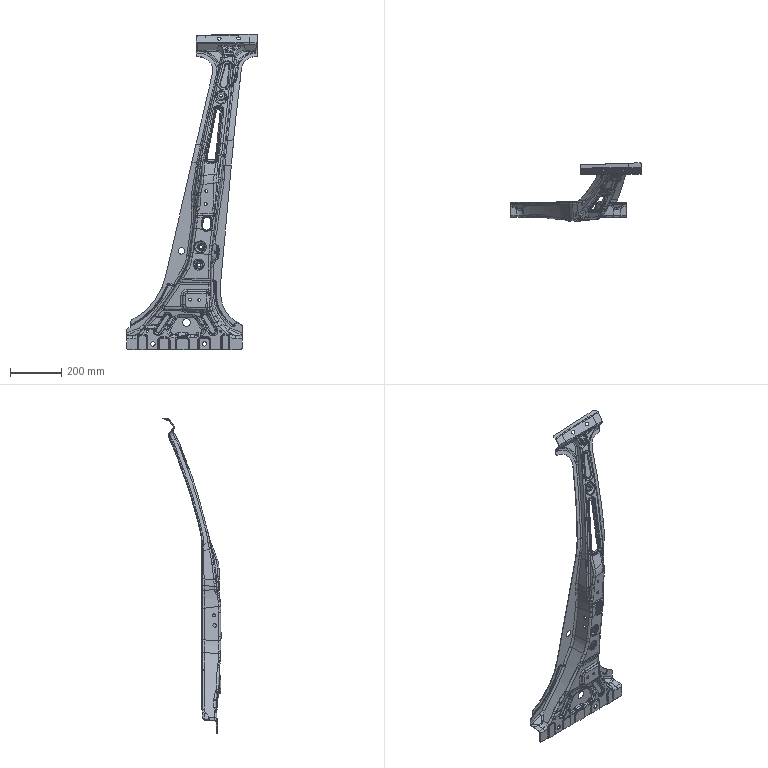Part | STEP file | FNA5401251 | 1 solid | 1668 faces | box 510.856 x 226.55 x 1230 mm | volume 703654 mm3 | spline 1242 | cylinder 269 | plane 107 | other 38 | sphere 10 | torus 2 | commonest cylinder face diameters 8 x42 12 x30 20 x24 16 x20 10 x17 14 x16